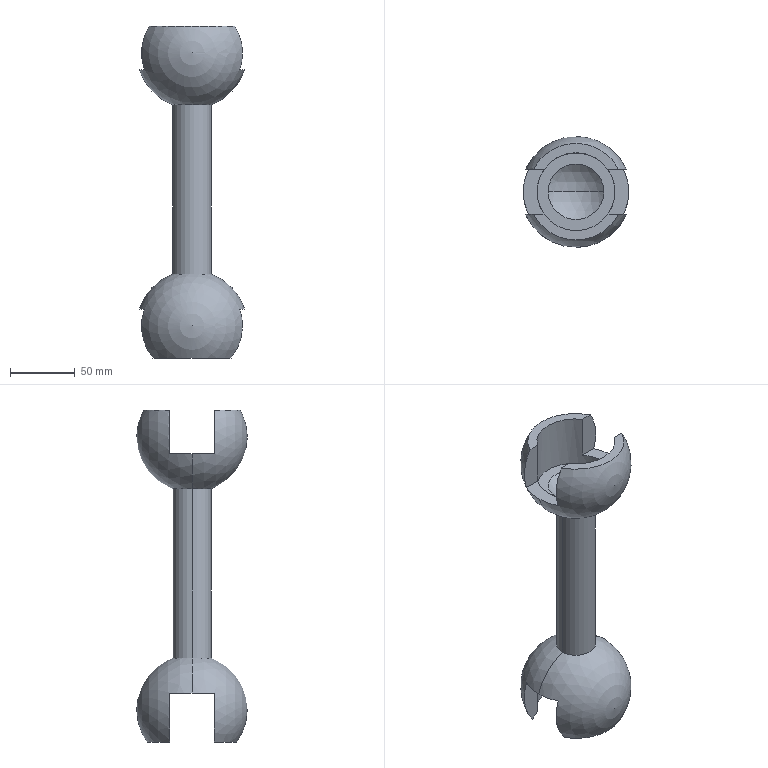Part | SolidWorks | features Chamfer 2, ICE 2, Extrusion 1, MirrorPattern 1, RevCut 1, Revolution 1 | 1 solid | 32 faces | box 80.921 x 85 x 255.451 mm | volume 326390 mm3 | plane 14 | sphere 8 | cylinder 6 | cone 4 | commonest cylinder face diameters 60 x4 30 x2
STEP:
#1=CARTESIAN_POINT('',(15.,0.,65.235));
#2=VERTEX_POINT('',#1);
#3=CARTESIAN_POINT('',(-15.,0.,65.235));
#4=VERTEX_POINT('',#3);
#5=CARTESIAN_POINT('',(0.,0.,65.235));
#6=DIRECTION('',(0.,0.,1.));
#7=DIRECTION('',(1.,0.,0.));
#8=AXIS2_PLACEMENT_3D('',#5,#6,#7);
#9=CIRCLE('',#8,15.);
#10=EDGE_CURVE('',#2,#4,#9,.T.);
#11=ORIENTED_EDGE('',*,*,#10,.T.);
#12=CARTESIAN_POINT('',(-40.46,0.,91.992));
#13=VERTEX_POINT('',#12);
#14=CARTESIAN_POINT('',(0.,0.,105.));
#15=DIRECTION('',(0.,1.,0.));
#16=DIRECTION('',(-1.,0.,0.));
#17=AXIS2_PLACEMENT_3D('',#14,#15,#16);
#18=CIRCLE('',#17,42.5);
#19=EDGE_CURVE('',#4,#13,#18,.T.);
#20=ORIENTED_EDGE('',*,*,#19,.T.);
#21=CARTESIAN_POINT('',(-36.62,17.204,91.992));
#22=VERTEX_POINT('',#21);
#23=CARTESIAN_POINT('',(0.,0.,91.992));
#24=DIRECTION('',(0.,0.,1.));
#25=DIRECTION('',(1.,0.,0.));
#26=AXIS2_PLACEMENT_3D('',#23,#24,#25);
#27=CIRCLE('',#26,40.46);
#28=EDGE_CURVE('',#22,#13,#27,.T.);
#29=ORIENTED_EDGE('',*,*,#28,.F.);
#30=CARTESIAN_POINT('',(-32.854,17.204,125.757));
#31=VERTEX_POINT('',#30);
#32=CARTESIAN_POINT('',(0.,17.204,105.));
#33=DIRECTION('',(0.,-1.,0.));
#34=DIRECTION('',(0.,0.,-1.));
#35=AXIS2_PLACEMENT_3D('',#32,#33,#34);
#36=CIRCLE('',#35,38.862);
#37=EDGE_CURVE('',#31,#22,#36,.T.);
#38=ORIENTED_EDGE('',*,*,#37,.F.);
#39=CARTESIAN_POINT('',(32.854,17.204,125.757));
#40=VERTEX_POINT('',#39);
#41=CARTESIAN_POINT('',(0.,0.,125.757));
#42=DIRECTION('',(0.,0.,-1.));
#43=DIRECTION('',(-1.,0.,0.));
#44=AXIS2_PLACEMENT_3D('',#41,#42,#43);
#45=CIRCLE('',#44,37.086);
#46=EDGE_CURVE('',#31,#40,#45,.T.);
#47=ORIENTED_EDGE('',*,*,#46,.T.);
#48=CARTESIAN_POINT('',(36.62,17.204,91.992));
#49=VERTEX_POINT('',#48);
#50=CARTESIAN_POINT('',(0.,17.204,105.));
#51=DIRECTION('',(0.,-1.,0.));
#52=DIRECTION('',(0.,0.,-1.));
#53=AXIS2_PLACEMENT_3D('',#50,#51,#52);
#54=CIRCLE('',#53,38.862);
#55=EDGE_CURVE('',#49,#40,#54,.T.);
#56=ORIENTED_EDGE('',*,*,#55,.F.);
#57=CARTESIAN_POINT('',(40.46,0.,91.992));
#58=VERTEX_POINT('',#57);
#59=CARTESIAN_POINT('',(0.,0.,91.992));
#60=DIRECTION('',(0.,0.,1.));
#61=DIRECTION('',(1.,0.,0.));
#62=AXIS2_PLACEMENT_3D('',#59,#60,#61);
#63=CIRCLE('',#62,40.46);
#64=EDGE_CURVE('',#58,#49,#63,.T.);
#65=ORIENTED_EDGE('',*,*,#64,.F.);
#66=CARTESIAN_POINT('',(0.,0.,105.));
#67=DIRECTION('',(0.,-1.,0.));
#68=DIRECTION('',(0.,0.,-1.));
#69=AXIS2_PLACEMENT_3D('',#66,#67,#68);
#70=CIRCLE('',#69,42.5);
#71=EDGE_CURVE('',#2,#58,#70,.T.);
#72=ORIENTED_EDGE('',*,*,#71,.F.);
#73=EDGE_LOOP('',(#11,#20,#29,#38,#47,#56,#65,#72));
#74=FACE_OUTER_BOUND('',#73,.T.);
#75=CARTESIAN_POINT('',(0.,0.,105.));
#76=DIRECTION('',(0.,1.,0.));
#77=DIRECTION('',(1.,0.,0.));
#78=AXIS2_PLACEMENT_3D('',#75,#76,#77);
#79=SPHERICAL_SURFACE('',#78,42.5);
#80=ADVANCED_FACE('',(#74),#79,.T.);
#81=CARTESIAN_POINT('',(0.,0.,-75.));
#82=VERTEX_POINT('',#81);
#83=CARTESIAN_POINT('',(-21.424,0.,-84.));
#84=VERTEX_POINT('',#83);
#85=CARTESIAN_POINT('',(0.,0.,-105.));
#86=DIRECTION('',(0.,-1.,0.));
#87=DIRECTION('',(0.,0.,-1.));
#88=AXIS2_PLACEMENT_3D('',#85,#86,#87);
#89=CIRCLE('',#88,30.);
#90=EDGE_CURVE('',#82,#84,#89,.T.);
#91=ORIENTED_EDGE('',*,*,#90,.F.);
#92=CARTESIAN_POINT('',(21.424,0.,-84.));
#93=VERTEX_POINT('',#92);
#94=CARTESIAN_POINT('',(0.,0.,-105.));
#95=DIRECTION('',(0.,1.,0.));
#96=DIRECTION('',(-1.,0.,0.));
#97=AXIS2_PLACEMENT_3D('',#94,#95,#96);
#98=CIRCLE('',#97,30.);
#99=EDGE_CURVE('',#82,#93,#98,.T.);
#100=ORIENTED_EDGE('',*,*,#99,.T.);
#101=CARTESIAN_POINT('',(0.,0.,-84.));
#102=DIRECTION('',(0.,0.,-1.));
#103=DIRECTION('',(1.,0.,0.));
#104=AXIS2_PLACEMENT_3D('',#101,#102,#103);
#105=CIRCLE('',#104,21.424);
#106=EDGE_CURVE('',#93,#84,#105,.T.);
#107=ORIENTED_EDGE('',*,*,#106,.T.);
#108=EDGE_LOOP('',(#91,#100,#107));
#109=FACE_OUTER_BOUND('',#108,.T.);
#110=CARTESIAN_POINT('',(0.,0.,-105.));
#111=DIRECTION('',(0.,1.,0.));
#112=DIRECTION('',(-1.,0.,0.));
#113=AXIS2_PLACEMENT_3D('',#110,#111,#112);
#114=SPHERICAL_SURFACE('',#113,30.);
#115=ADVANCED_FACE('',(#109),#114,.F.);
#116=CARTESIAN_POINT('',(15.,0.,-65.235));
#117=VERTEX_POINT('',#116);
#118=CARTESIAN_POINT('',(-15.,0.,-65.235));
#119=VERTEX_POINT('',#118);
#120=CARTESIAN_POINT('',(0.,0.,-65.235));
#121=DIRECTION('',(0.,0.,-1.));
#122=DIRECTION('',(-1.,0.,0.));
#123=AXIS2_PLACEMENT_3D('',#120,#121,#122);
#124=CIRCLE('',#123,15.);
#125=EDGE_CURVE('',#117,#119,#124,.T.);
#126=ORIENTED_EDGE('',*,*,#125,.T.);
#127=CARTESIAN_POINT('',(-40.46,0.,-91.992));
#128=VERTEX_POINT('',#127);
#129=CARTESIAN_POINT('',(0.,0.,-105.));
#130=DIRECTION('',(0.,-1.,0.));
#131=DIRECTION('',(1.,0.,0.));
#132=AXIS2_PLACEMENT_3D('',#129,#130,#131);
#133=CIRCLE('',#132,42.5);
#134=EDGE_CURVE('',#119,#128,#133,.T.);
#135=ORIENTED_EDGE('',*,*,#134,.T.);
#136=CARTESIAN_POINT('',(-36.62,-17.204,-91.992));
#137=VERTEX_POINT('',#136);
#138=CARTESIAN_POINT('',(0.,0.,-91.992));
#139=DIRECTION('',(0.,0.,1.));
#140=DIRECTION('',(1.,0.,0.));
#141=AXIS2_PLACEMENT_3D('',#138,#139,#140);
#142=CIRCLE('',#141,40.46);
#143=EDGE_CURVE('',#128,#137,#142,.T.);
#144=ORIENTED_EDGE('',*,*,#143,.T.);
#145=CARTESIAN_POINT('',(-30.008,-17.204,-129.694));
#146=VERTEX_POINT('',#145);
#147=CARTESIAN_POINT('',(0.,-17.204,-105.));
#148=DIRECTION('',(0.,1.,0.));
#149=DIRECTION('',(0.,0.,1.));
#150=AXIS2_PLACEMENT_3D('',#147,#148,#149);
#151=CIRCLE('',#150,38.862);
#152=EDGE_CURVE('',#146,#137,#151,.T.);
#153=ORIENTED_EDGE('',*,*,#152,.F.);
#154=CARTESIAN_POINT('',(30.008,-17.204,-129.694));
#155=VERTEX_POINT('',#154);
#156=CARTESIAN_POINT('',(0.,0.,-129.694));
#157=DIRECTION('',(0.,0.,1.));
#158=DIRECTION('',(1.,0.,0.));
#159=AXIS2_PLACEMENT_3D('',#156,#157,#158);
#160=CIRCLE('',#159,34.59);
#161=EDGE_CURVE('',#146,#155,#160,.T.);
#162=ORIENTED_EDGE('',*,*,#161,.T.);
#163=CARTESIAN_POINT('',(36.62,-17.204,-91.992));
#164=VERTEX_POINT('',#163);
#165=CARTESIAN_POINT('',(0.,-17.204,-105.));
#166=DIRECTION('',(0.,1.,0.));
#167=DIRECTION('',(0.,0.,1.));
#168=AXIS2_PLACEMENT_3D('',#165,#166,#167);
#169=CIRCLE('',#168,38.862);
#170=EDGE_CURVE('',#164,#155,#169,.T.);
#171=ORIENTED_EDGE('',*,*,#170,.F.);
#172=CARTESIAN_POINT('',(40.46,0.,-91.992));
#173=VERTEX_POINT('',#172);
#174=CARTESIAN_POINT('',(0.,0.,-91.992));
#175=DIRECTION('',(0.,0.,1.));
#176=DIRECTION('',(1.,0.,0.));
#177=AXIS2_PLACEMENT_3D('',#174,#175,#176);
#178=CIRCLE('',#177,40.46);
#179=EDGE_CURVE('',#164,#173,#178,.T.);
#180=ORIENTED_EDGE('',*,*,#179,.T.);
#181=CARTESIAN_POINT('',(0.,0.,-105.));
#182=DIRECTION('',(0.,1.,0.));
#183=DIRECTION('',(0.,0.,1.));
#184=AXIS2_PLACEMENT_3D('',#181,#182,#183);
#185=CIRCLE('',#184,42.5);
#186=EDGE_CURVE('',#117,#173,#185,.T.);
#187=ORIENTED_EDGE('',*,*,#186,.F.);
#188=EDGE_LOOP('',(#126,#135,#144,#153,#162,#171,#180,#187));
#189=FACE_OUTER_BOUND('',#188,.T.);
#190=CARTESIAN_POINT('',(0.,0.,-105.));
#191=DIRECTION('',(0.,-1.,0.));
#192=DIRECTION('',(1.,0.,0.));
#193=AXIS2_PLACEMENT_3D('',#190,#191,#192);
#194=SPHERICAL_SURFACE('',#193,42.5);
#195=ADVANCED_FACE('',(#189),#194,.T.);
#196=CARTESIAN_POINT('',(-30.,0.,-84.));
#197=VERTEX_POINT('',#196);
#198=CARTESIAN_POINT('',(30.,0.,-84.));
#199=VERTEX_POINT('',#198);
#200=CARTESIAN_POINT('',(0.,0.,-84.));
#201=DIRECTION('',(0.,0.,1.));
#202=DIRECTION('',(1.,0.,0.));
#203=AXIS2_PLACEMENT_3D('',#200,#201,#202);
#204=CIRCLE('',#203,30.);
#205=EDGE_CURVE('',#197,#199,#204,.T.);
#206=ORIENTED_EDGE('',*,*,#205,.T.);
#207=CARTESIAN_POINT('',(30.,0.,-91.992));
#208=VERTEX_POINT('',#207);
#209=CARTESIAN_POINT('',(30.,0.,-84.));
#210=DIRECTION('',(0.,0.,-1.));
#211=VECTOR('',#210,1000.);
#212=LINE('',#209,#211);
#213=EDGE_CURVE('',#199,#208,#212,.T.);
#214=ORIENTED_EDGE('',*,*,#213,.T.);
#215=CARTESIAN_POINT('',(24.577,-17.204,-91.992));
#216=VERTEX_POINT('',#215);
#217=CARTESIAN_POINT('',(0.,0.,-91.992));
#218=DIRECTION('',(0.,0.,1.));
#219=DIRECTION('',(1.,0.,0.));
#220=AXIS2_PLACEMENT_3D('',#217,#218,#219);
#221=CIRCLE('',#220,30.);
#222=EDGE_CURVE('',#216,#208,#221,.T.);
#223=ORIENTED_EDGE('',*,*,#222,.F.);
#224=CARTESIAN_POINT('',(24.577,-17.204,-125.104));
#225=VERTEX_POINT('',#224);
#226=CARTESIAN_POINT('',(24.577,-17.204,-84.));
#227=DIRECTION('',(0.,0.,-1.));
#228=VECTOR('',#227,1000.);
#229=LINE('',#226,#228);
#230=EDGE_CURVE('',#216,#225,#229,.T.);
#231=ORIENTED_EDGE('',*,*,#230,.T.);
#232=CARTESIAN_POINT('',(-24.577,-17.204,-125.104));
#233=VERTEX_POINT('',#232);
#234=CARTESIAN_POINT('',(0.,0.,-125.104));
#235=DIRECTION('',(0.,0.,-1.));
#236=DIRECTION('',(1.,0.,0.));
#237=AXIS2_PLACEMENT_3D('',#234,#235,#236);
#238=CIRCLE('',#237,30.);
#239=EDGE_CURVE('',#225,#233,#238,.T.);
#240=ORIENTED_EDGE('',*,*,#239,.T.);
#241=CARTESIAN_POINT('',(-24.577,-17.204,-91.992));
#242=VERTEX_POINT('',#241);
#243=CARTESIAN_POINT('',(-24.577,-17.204,-84.));
#244=DIRECTION('',(0.,0.,1.));
#245=VECTOR('',#244,1000.);
#246=LINE('',#243,#245);
#247=EDGE_CURVE('',#233,#242,#246,.T.);
#248=ORIENTED_EDGE('',*,*,#247,.T.);
#249=CARTESIAN_POINT('',(-30.,0.,-91.992));
#250=VERTEX_POINT('',#249);
#251=CARTESIAN_POINT('',(0.,0.,-91.992));
#252=DIRECTION('',(0.,0.,1.));
#253=DIRECTION('',(1.,0.,0.));
#254=AXIS2_PLACEMENT_3D('',#251,#252,#253);
#255=CIRCLE('',#254,30.);
#256=EDGE_CURVE('',#250,#242,#255,.T.);
#257=ORIENTED_EDGE('',*,*,#256,.F.);
#258=CARTESIAN_POINT('',(-30.,0.,-84.));
#259=DIRECTION('',(0.,0.,-1.));
#260=VECTOR('',#259,1000.);
#261=LINE('',#258,#260);
#262=EDGE_CURVE('',#197,#250,#261,.T.);
#263=ORIENTED_EDGE('',*,*,#262,.F.);
#264=EDGE_LOOP('',(#206,#214,#223,#231,#240,#248,#257,#263));
#265=FACE_OUTER_BOUND('',#264,.T.);
#266=CARTESIAN_POINT('',(0.,0.,-84.));
#267=DIRECTION('',(0.,0.,-1.));
#268=DIRECTION('',(-1.,0.,0.));
#269=AXIS2_PLACEMENT_3D('',#266,#267,#268);
#270=CYLINDRICAL_SURFACE('',#269,30.);
#271=ADVANCED_FACE('',(#265),#270,.F.);
#272=ORIENTED_EDGE('',*,*,#10,.F.);
#273=CARTESIAN_POINT('',(15.,0.,80.));
#274=DIRECTION('',(0.,0.,-1.));
#275=VECTOR('',#274,1000.);
#276=LINE('',#273,#275);
#277=EDGE_CURVE('',#2,#117,#276,.T.);
#278=ORIENTED_EDGE('',*,*,#277,.T.);
#279=CARTESIAN_POINT('',(0.,0.,-65.235));
#280=DIRECTION('',(0.,0.,-1.));
#281=DIRECTION('',(-1.,0.,0.));
#282=AXIS2_PLACEMENT_3D('',#279,#280,#281);
#283=CIRCLE('',#282,15.);
#284=EDGE_CURVE('',#119,#117,#283,.T.);
#285=ORIENTED_EDGE('',*,*,#284,.F.);
#286=CARTESIAN_POINT('',(-15.,0.,80.));
#287=DIRECTION('',(0.,0.,-1.));
#288=VECTOR('',#287,1000.);
#289=LINE('',#286,#288);
#290=EDGE_CURVE('',#4,#119,#289,.T.);
#291=ORIENTED_EDGE('',*,*,#290,.F.);
#292=EDGE_LOOP('',(#272,#278,#285,#291));
#293=FACE_OUTER_BOUND('',#292,.T.);
#294=CARTESIAN_POINT('',(0.,0.,80.));
#295=DIRECTION('',(0.,0.,-1.));
#296=DIRECTION('',(-1.,0.,0.));
#297=AXIS2_PLACEMENT_3D('',#294,#295,#296);
#298=CYLINDRICAL_SURFACE('',#297,15.);
#299=ADVANCED_FACE('',(#293),#298,.T.);
#300=CARTESIAN_POINT('',(-30.,0.,84.));
#301=VERTEX_POINT('',#300);
#302=CARTESIAN_POINT('',(30.,0.,84.));
#303=VERTEX_POINT('',#302);
#304=CARTESIAN_POINT('',(0.,0.,84.));
#305=DIRECTION('',(0.,0.,1.));
#306=DIRECTION('',(1.,0.,0.));
#307=AXIS2_PLACEMENT_3D('',#304,#305,#306);
#308=CIRCLE('',#307,30.);
#309=EDGE_CURVE('',#301,#303,#308,.T.);
#310=ORIENTED_EDGE('',*,*,#309,.F.);
#311=CARTESIAN_POINT('',(-30.,0.,91.992));
#312=VERTEX_POINT('',#311);
#313=CARTESIAN_POINT('',(-30.,0.,84.));
#314=DIRECTION('',(0.,0.,1.));
#315=VECTOR('',#314,1000.);
#316=LINE('',#313,#315);
#317=EDGE_CURVE('',#301,#312,#316,.T.);
#318=ORIENTED_EDGE('',*,*,#317,.T.);
#319=CARTESIAN_POINT('',(-24.577,-17.204,91.992));
#320=VERTEX_POINT('',#319);
#321=CARTESIAN_POINT('',(0.,0.,91.992));
#322=DIRECTION('',(0.,0.,-1.));
#323=DIRECTION('',(1.,0.,0.));
#324=AXIS2_PLACEMENT_3D('',#321,#322,#323);
#325=CIRCLE('',#324,30.);
#326=EDGE_CURVE('',#320,#312,#325,.T.);
#327=ORIENTED_EDGE('',*,*,#326,.F.);
#328=CARTESIAN_POINT('',(-24.577,-17.204,125.749));
#329=VERTEX_POINT('',#328);
#330=CARTESIAN_POINT('',(-24.577,-17.204,84.));
#331=DIRECTION('',(0.,0.,1.));
#332=VECTOR('',#331,1000.);
#333=LINE('',#330,#332);
#334=EDGE_CURVE('',#320,#329,#333,.T.);
#335=ORIENTED_EDGE('',*,*,#334,.T.);
#336=CARTESIAN_POINT('',(24.577,-17.204,125.749));
#337=VERTEX_POINT('',#336);
#338=CARTESIAN_POINT('',(0.,0.,125.749));
#339=DIRECTION('',(0.,0.,1.));
#340=DIRECTION('',(-1.,0.,0.));
#341=AXIS2_PLACEMENT_3D('',#338,#339,#340);
#342=CIRCLE('',#341,30.);
#343=EDGE_CURVE('',#329,#337,#342,.T.);
#344=ORIENTED_EDGE('',*,*,#343,.T.);
#345=CARTESIAN_POINT('',(24.577,-17.204,91.992));
#346=VERTEX_POINT('',#345);
#347=CARTESIAN_POINT('',(24.577,-17.204,84.));
#348=DIRECTION('',(0.,0.,-1.));
#349=VECTOR('',#348,1000.);
#350=LINE('',#347,#349);
#351=EDGE_CURVE('',#337,#346,#350,.T.);
#352=ORIENTED_EDGE('',*,*,#351,.T.);
#353=CARTESIAN_POINT('',(30.,0.,91.992));
#354=VERTEX_POINT('',#353);
#355=CARTESIAN_POINT('',(0.,0.,91.992));
#356=DIRECTION('',(0.,0.,-1.));
#357=DIRECTION('',(1.,0.,0.));
#358=AXIS2_PLACEMENT_3D('',#355,#356,#357);
#359=CIRCLE('',#358,30.);
#360=EDGE_CURVE('',#354,#346,#359,.T.);
#361=ORIENTED_EDGE('',*,*,#360,.F.);
#362=CARTESIAN_POINT('',(30.,0.,84.));
#363=DIRECTION('',(0.,0.,1.));
#364=VECTOR('',#363,1000.);
#365=LINE('',#362,#364);
#366=EDGE_CURVE('',#303,#354,#365,.T.);
#367=ORIENTED_EDGE('',*,*,#366,.F.);
#368=EDGE_LOOP('',(#310,#318,#327,#335,#344,#352,#361,#367));
#369=FACE_OUTER_BOUND('',#368,.T.);
#370=CARTESIAN_POINT('',(0.,0.,84.));
#371=DIRECTION('',(0.,0.,1.));
#372=DIRECTION('',(1.,0.,0.));
#373=AXIS2_PLACEMENT_3D('',#370,#371,#372);
#374=CYLINDRICAL_SURFACE('',#373,30.);
#375=ADVANCED_FACE('',(#369),#374,.F.);
#376=CARTESIAN_POINT('',(0.,0.,75.));
#377=VERTEX_POINT('',#376);
#378=CARTESIAN_POINT('',(-21.424,0.,84.));
#379=VERTEX_POINT('',#378);
#380=CARTESIAN_POINT('',(0.,0.,105.));
#381=DIRECTION('',(0.,1.,0.));
#382=DIRECTION('',(0.,0.,1.));
#383=AXIS2_PLACEMENT_3D('',#380,#381,#382);
#384=CIRCLE('',#383,30.);
#385=EDGE_CURVE('',#377,#379,#384,.T.);
#386=ORIENTED_EDGE('',*,*,#385,.F.);
#387=CARTESIAN_POINT('',(21.424,0.,84.));
#388=VERTEX_POINT('',#387);
#389=CARTESIAN_POINT('',(0.,0.,105.));
#390=DIRECTION('',(0.,-1.,0.));
#391=DIRECTION('',(1.,0.,0.));
#392=AXIS2_PLACEMENT_3D('',#389,#390,#391);
#393=CIRCLE('',#392,30.);
#394=EDGE_CURVE('',#377,#388,#393,.T.);
#395=ORIENTED_EDGE('',*,*,#394,.T.);
#396=CARTESIAN_POINT('',(0.,0.,84.));
#397=DIRECTION('',(0.,0.,1.));
#398=DIRECTION('',(-1.,0.,0.));
#399=AXIS2_PLACEMENT_3D('',#396,#397,#398);
#400=CIRCLE('',#399,21.424);
#401=EDGE_CURVE('',#388,#379,#400,.T.);
#402=ORIENTED_EDGE('',*,*,#401,.T.);
#403=EDGE_LOOP('',(#386,#395,#402));
#404=FACE_OUTER_BOUND('',#403,.T.);
#405=CARTESIAN_POINT('',(0.,0.,105.));
#406=DIRECTION('',(0.,-1.,0.));
#407=DIRECTION('',(-1.,0.,0.));
#408=AXIS2_PLACEMENT_3D('',#405,#406,#407);
#409=SPHERICAL_SURFACE('',#408,30.);
#410=ADVANCED_FACE('',(#404),#409,.F.);
#411=ORIENTED_EDGE('',*,*,#394,.F.);
#412=ORIENTED_EDGE('',*,*,#385,.T.);
#413=CARTESIAN_POINT('',(0.,0.,84.));
#414=DIRECTION('',(0.,0.,1.));
#415=DIRECTION('',(-1.,0.,0.));
#416=AXIS2_PLACEMENT_3D('',#413,#414,#415);
#417=CIRCLE('',#416,21.424);
#418=EDGE_CURVE('',#379,#388,#417,.T.);
#419=ORIENTED_EDGE('',*,*,#418,.T.);
#420=EDGE_LOOP('',(#411,#412,#419));
#421=FACE_OUTER_BOUND('',#420,.T.);
#422=CARTESIAN_POINT('',(0.,0.,105.));
#423=DIRECTION('',(0.,-1.,0.));
#424=DIRECTION('',(-1.,0.,0.));
#425=AXIS2_PLACEMENT_3D('',#422,#423,#424);
#426=SPHERICAL_SURFACE('',#425,30.);
#427=ADVANCED_FACE('',(#421),#426,.F.);
#428=ORIENTED_EDGE('',*,*,#317,.F.);
#429=CARTESIAN_POINT('',(0.,0.,84.));
#430=DIRECTION('',(0.,0.,1.));
#431=DIRECTION('',(1.,0.,0.));
#432=AXIS2_PLACEMENT_3D('',#429,#430,#431);
#433=CIRCLE('',#432,30.);
#434=EDGE_CURVE('',#303,#301,#433,.T.);
#435=ORIENTED_EDGE('',*,*,#434,.F.);
#436=ORIENTED_EDGE('',*,*,#366,.T.);
#437=CARTESIAN_POINT('',(24.577,17.204,91.992));
#438=VERTEX_POINT('',#437);
#439=CARTESIAN_POINT('',(0.,0.,91.992));
#440=DIRECTION('',(0.,0.,-1.));
#441=DIRECTION('',(1.,0.,0.));
#442=AXIS2_PLACEMENT_3D('',#439,#440,#441);
#443=CIRCLE('',#442,30.);
#444=EDGE_CURVE('',#438,#354,#443,.T.);
#445=ORIENTED_EDGE('',*,*,#444,.F.);
#446=CARTESIAN_POINT('',(24.577,17.204,125.749));
#447=VERTEX_POINT('',#446);
#448=CARTESIAN_POINT('',(24.577,17.204,84.));
#449=DIRECTION('',(0.,0.,-1.));
#450=VECTOR('',#449,1000.);
#451=LINE('',#448,#450);
#452=EDGE_CURVE('',#447,#438,#451,.T.);
#453=ORIENTED_EDGE('',*,*,#452,.F.);
#454=CARTESIAN_POINT('',(-24.577,17.204,125.749));
#455=VERTEX_POINT('',#454);
#456=CARTESIAN_POINT('',(0.,0.,125.749));
#457=DIRECTION('',(0.,0.,1.));
#458=DIRECTION('',(-1.,0.,0.));
#459=AXIS2_PLACEMENT_3D('',#456,#457,#458);
#460=CIRCLE('',#459,30.);
#461=EDGE_CURVE('',#447,#455,#460,.T.);
#462=ORIENTED_EDGE('',*,*,#461,.T.);
#463=CARTESIAN_POINT('',(-24.577,17.204,91.992));
#464=VERTEX_POINT('',#463);
#465=CARTESIAN_POINT('',(-24.577,17.204,84.));
#466=DIRECTION('',(0.,0.,1.));
#467=VECTOR('',#466,1000.);
#468=LINE('',#465,#467);
#469=EDGE_CURVE('',#464,#455,#468,.T.);
#470=ORIENTED_EDGE('',*,*,#469,.F.);
#471=CARTESIAN_POINT('',(0.,0.,91.992));
#472=DIRECTION('',(0.,0.,-1.));
#473=DIRECTION('',(1.,0.,0.));
#474=AXIS2_PLACEMENT_3D('',#471,#472,#473);
#475=CIRCLE('',#474,30.);
#476=EDGE_CURVE('',#312,#464,#475,.T.);
#477=ORIENTED_EDGE('',*,*,#476,.F.);
#478=EDGE_LOOP('',(#428,#435,#436,#445,#453,#462,#470,#477));
#479=FACE_OUTER_BOUND('',#478,.T.);
#480=CARTESIAN_POINT('',(0.,0.,84.));
#481=DIRECTION('',(0.,0.,1.));
#482=DIRECTION('',(1.,0.,0.));
#483=AXIS2_PLACEMENT_3D('',#480,#481,#482);
#484=CYLINDRICAL_SURFACE('',#483,30.);
#485=ADVANCED_FACE('',(#479),#484,.F.);
#486=ORIENTED_EDGE('',*,*,#434,.T.);
#487=ORIENTED_EDGE('',*,*,#309,.T.);
#488=EDGE_LOOP('',(#486,#487));
#489=FACE_OUTER_BOUND('',#488,.T.);
#490=ORIENTED_EDGE('',*,*,#418,.F.);
#491=ORIENTED_EDGE('',*,*,#401,.F.);
#492=EDGE_LOOP('',(#490,#491));
#493=FACE_BOUND('',#492,.T.);
#494=CARTESIAN_POINT('',(0.,0.,84.));
#495=DIRECTION('',(0.,0.,-1.));
#496=DIRECTION('',(1.,0.,0.));
#497=AXIS2_PLACEMENT_3D('',#494,#495,#496);
#498=PLANE('',#497);
#499=ADVANCED_FACE('',(#489,#493),#498,.F.);
#500=ORIENTED_EDGE('',*,*,#277,.F.);
#501=CARTESIAN_POINT('',(0.,0.,65.235));
#502=DIRECTION('',(0.,0.,1.));
#503=DIRECTION('',(1.,0.,0.));
#504=AXIS2_PLACEMENT_3D('',#501,#502,#503);
#505=CIRCLE('',#504,15.);
#506=EDGE_CURVE('',#4,#2,#505,.T.);
#507=ORIENTED_EDGE('',*,*,#506,.F.);
#508=ORIENTED_EDGE('',*,*,#290,.T.);
#509=ORIENTED_EDGE('',*,*,#125,.F.);
#510=EDGE_LOOP('',(#500,#507,#508,#509));
#511=FACE_OUTER_BOUND('',#510,.T.);
#512=CARTESIAN_POINT('',(0.,0.,80.));
#513=DIRECTION('',(0.,0.,-1.));
#514=DIRECTION('',(-1.,0.,0.));
#515=AXIS2_PLACEMENT_3D('',#512,#513,#514);
#516=CYLINDRICAL_SURFACE('',#515,15.);
#517=ADVANCED_FACE('',(#511),#516,.T.);
#518=ORIENTED_EDGE('',*,*,#213,.F.);
#519=CARTESIAN_POINT('',(0.,0.,-84.));
#520=DIRECTION('',(0.,0.,1.));
#521=DIRECTION('',(1.,0.,0.));
#522=AXIS2_PLACEMENT_3D('',#519,#520,#521);
#523=CIRCLE('',#522,30.);
#524=EDGE_CURVE('',#199,#197,#523,.T.);
#525=ORIENTED_EDGE('',*,*,#524,.T.);
#526=ORIENTED_EDGE('',*,*,#262,.T.);
#527=CARTESIAN_POINT('',(-24.577,17.204,-91.992));
#528=VERTEX_POINT('',#527);
#529=CARTESIAN_POINT('',(0.,0.,-91.992));
#530=DIRECTION('',(0.,0.,1.));
#531=DIRECTION('',(1.,0.,0.));
#532=AXIS2_PLACEMENT_3D('',#529,#530,#531);
#533=CIRCLE('',#532,30.);
#534=EDGE_CURVE('',#528,#250,#533,.T.);
#535=ORIENTED_EDGE('',*,*,#534,.F.);
#536=CARTESIAN_POINT('',(-24.577,17.204,-125.104));
#537=VERTEX_POINT('',#536);
#538=CARTESIAN_POINT('',(-24.577,17.204,-84.));
#539=DIRECTION('',(0.,0.,1.));
#540=VECTOR('',#539,1000.);
#541=LINE('',#538,#540);
#542=EDGE_CURVE('',#537,#528,#541,.T.);
#543=ORIENTED_EDGE('',*,*,#542,.F.);
#544=CARTESIAN_POINT('',(24.577,17.204,-125.104));
#545=VERTEX_POINT('',#544);
#546=CARTESIAN_POINT('',(0.,0.,-125.104));
#547=DIRECTION('',(0.,0.,-1.));
#548=DIRECTION('',(1.,0.,0.));
#549=AXIS2_PLACEMENT_3D('',#546,#547,#548);
#550=CIRCLE('',#549,30.);
#551=EDGE_CURVE('',#537,#545,#550,.T.);
#552=ORIENTED_EDGE('',*,*,#551,.T.);
#553=CARTESIAN_POINT('',(24.577,17.204,-91.992));
#554=VERTEX_POINT('',#553);
#555=CARTESIAN_POINT('',(24.577,17.204,-84.));
#556=DIRECTION('',(0.,0.,-1.));
#557=VECTOR('',#556,1000.);
#558=LINE('',#555,#557);
#559=EDGE_CURVE('',#554,#545,#558,.T.);
#560=ORIENTED_EDGE('',*,*,#559,.F.);
#561=CARTESIAN_POINT('',(0.,0.,-91.992));
#562=DIRECTION('',(0.,0.,1.));
#563=DIRECTION('',(1.,0.,0.));
#564=AXIS2_PLACEMENT_3D('',#561,#562,#563);
#565=CIRCLE('',#564,30.);
#566=EDGE_CURVE('',#208,#554,#565,.T.);
#567=ORIENTED_EDGE('',*,*,#566,.F.);
#568=EDGE_LOOP('',(#518,#525,#526,#535,#543,#552,#560,#567));
#569=FACE_OUTER_BOUND('',#568,.T.);
#570=CARTESIAN_POINT('',(0.,0.,-84.));
#571=DIRECTION('',(0.,0.,-1.));
#572=DIRECTION('',(-1.,0.,0.));
#573=AXIS2_PLACEMENT_3D('',#570,#571,#572);
#574=CYLINDRICAL_SURFACE('',#573,30.);
#575=ADVANCED_FACE('',(#569),#574,.F.);
#576=ORIENTED_EDGE('',*,*,#134,.F.);
#577=ORIENTED_EDGE('',*,*,#284,.T.);
#578=ORIENTED_EDGE('',*,*,#186,.T.);
#579=CARTESIAN_POINT('',(36.62,17.204,-91.992));
#580=VERTEX_POINT('',#579);
#581=CARTESIAN_POINT('',(0.,0.,-91.992));
#582=DIRECTION('',(0.,0.,1.));
#583=DIRECTION('',(1.,0.,0.));
#584=AXIS2_PLACEMENT_3D('',#581,#582,#583);
#585=CIRCLE('',#584,40.46);
#586=EDGE_CURVE('',#173,#580,#585,.T.);
#587=ORIENTED_EDGE('',*,*,#586,.T.);
#588=CARTESIAN_POINT('',(30.008,17.204,-129.694));
#589=VERTEX_POINT('',#588);
#590=CARTESIAN_POINT('',(0.,17.204,-105.));
#591=DIRECTION('',(0.,1.,0.));
#592=DIRECTION('',(0.,0.,1.));
#593=AXIS2_PLACEMENT_3D('',#590,#591,#592);
#594=CIRCLE('',#593,38.862);
#595=EDGE_CURVE('',#580,#589,#594,.T.);
#596=ORIENTED_EDGE('',*,*,#595,.T.);
#597=CARTESIAN_POINT('',(-30.008,17.204,-129.694));
#598=VERTEX_POINT('',#597);
#599=CARTESIAN_POINT('',(0.,0.,-129.694));
#600=DIRECTION('',(0.,0.,1.));
#601=DIRECTION('',(1.,0.,0.));
#602=AXIS2_PLACEMENT_3D('',#599,#600,#601);
#603=CIRCLE('',#602,34.59);
#604=EDGE_CURVE('',#589,#598,#603,.T.);
#605=ORIENTED_EDGE('',*,*,#604,.T.);
#606=CARTESIAN_POINT('',(-36.62,17.204,-91.992));
#607=VERTEX_POINT('',#606);
#608=CARTESIAN_POINT('',(0.,17.204,-105.));
#609=DIRECTION('',(0.,1.,0.));
#610=DIRECTION('',(0.,0.,1.));
#611=AXIS2_PLACEMENT_3D('',#608,#609,#610);
#612=CIRCLE('',#611,38.862);
#613=EDGE_CURVE('',#598,#607,#612,.T.);
#614=ORIENTED_EDGE('',*,*,#613,.T.);
#615=CARTESIAN_POINT('',(0.,0.,-91.992));
#616=DIRECTION('',(0.,0.,1.));
#617=DIRECTION('',(1.,0.,0.));
#618=AXIS2_PLACEMENT_3D('',#615,#616,#617);
#619=CIRCLE('',#618,40.46);
#620=EDGE_CURVE('',#607,#128,#619,.T.);
#621=ORIENTED_EDGE('',*,*,#620,.T.);
#622=EDGE_LOOP('',(#576,#577,#578,#587,#596,#605,#614,#621));
#623=FACE_OUTER_BOUND('',#622,.T.);
#624=CARTESIAN_POINT('',(0.,0.,-105.));
#625=DIRECTION('',(0.,-1.,0.));
#626=DIRECTION('',(1.,0.,0.));
#627=AXIS2_PLACEMENT_3D('',#624,#625,#626);
#628=SPHERICAL_SURFACE('',#627,42.5);
#629=ADVANCED_FACE('',(#623),#628,.T.);
#630=ORIENTED_EDGE('',*,*,#99,.F.);
#631=ORIENTED_EDGE('',*,*,#90,.T.);
#632=CARTESIAN_POINT('',(0.,0.,-84.));
#633=DIRECTION('',(0.,0.,-1.));
#634=DIRECTION('',(1.,0.,0.));
#635=AXIS2_PLACEMENT_3D('',#632,#633,#634);
#636=CIRCLE('',#635,21.424);
#637=EDGE_CURVE('',#84,#93,#636,.T.);
#638=ORIENTED_EDGE('',*,*,#637,.T.);
#639=EDGE_LOOP('',(#630,#631,#638));
#640=FACE_OUTER_BOUND('',#639,.T.);
#641=CARTESIAN_POINT('',(0.,0.,-105.));
#642=DIRECTION('',(0.,1.,0.));
#643=DIRECTION('',(-1.,0.,0.));
#644=AXIS2_PLACEMENT_3D('',#641,#642,#643);
#645=SPHERICAL_SURFACE('',#644,30.);
#646=ADVANCED_FACE('',(#640),#645,.F.);
#647=ORIENTED_EDGE('',*,*,#205,.F.);
#648=ORIENTED_EDGE('',*,*,#524,.F.);
#649=EDGE_LOOP('',(#647,#648));
#650=FACE_OUTER_BOUND('',#649,.T.);
#651=ORIENTED_EDGE('',*,*,#637,.F.);
#652=ORIENTED_EDGE('',*,*,#106,.F.);
#653=EDGE_LOOP('',(#651,#652));
#654=FACE_BOUND('',#653,.T.);
#655=CARTESIAN_POINT('',(0.,0.,-84.));
#656=DIRECTION('',(0.,0.,1.));
#657=DIRECTION('',(1.,0.,0.));
#658=AXIS2_PLACEMENT_3D('',#655,#656,#657);
#659=PLANE('',#658);
#660=ADVANCED_FACE('',(#650,#654),#659,.F.);
#661=ORIENTED_EDGE('',*,*,#613,.F.);
#662=CARTESIAN_POINT('',(-30.008,17.204,-129.694));
#663=CARTESIAN_POINT('',(-28.217,17.204,-128.14));
#664=CARTESIAN_POINT('',(-26.411,17.204,-126.606));
#665=CARTESIAN_POINT('',(-24.577,17.204,-125.104));
#666=B_SPLINE_CURVE_WITH_KNOTS('',3,(#662,#663,#664,#665),.UNSPECIFIED.,.F.,.F.,(4,4),(0.,0.007111),.UNSPECIFIED.);
#667=EDGE_CURVE('',#598,#537,#666,.T.);
#668=ORIENTED_EDGE('',*,*,#667,.T.);
#669=ORIENTED_EDGE('',*,*,#542,.T.);
#670=CARTESIAN_POINT('',(-75.5,17.204,-91.992));
#671=DIRECTION('',(1.,0.,0.));
#672=VECTOR('',#671,1000.);
#673=LINE('',#670,#672);
#674=EDGE_CURVE('',#607,#528,#673,.T.);
#675=ORIENTED_EDGE('',*,*,#674,.F.);
#676=EDGE_LOOP('',(#661,#668,#669,#675));
#677=FACE_OUTER_BOUND('',#676,.T.);
#678=CARTESIAN_POINT('',(-75.5,17.204,-178.216));
#679=DIRECTION('',(0.,1.,0.));
#680=DIRECTION('',(0.,0.,1.));
#681=AXIS2_PLACEMENT_3D('',#678,#679,#680);
#682=PLANE('',#681);
#683=ADVANCED_FACE('',(#677),#682,.F.);
#684=ORIENTED_EDGE('',*,*,#534,.T.);
#685=ORIENTED_EDGE('',*,*,#256,.T.);
#686=CARTESIAN_POINT('',(-75.5,-17.204,-91.992));
#687=DIRECTION('',(1.,0.,0.));
#688=VECTOR('',#687,1000.);
#689=LINE('',#686,#688);
#690=EDGE_CURVE('',#137,#242,#689,.T.);
#691=ORIENTED_EDGE('',*,*,#690,.F.);
#692=ORIENTED_EDGE('',*,*,#143,.F.);
#693=ORIENTED_EDGE('',*,*,#620,.F.);
#694=ORIENTED_EDGE('',*,*,#674,.T.);
#695=EDGE_LOOP('',(#684,#685,#691,#692,#693,#694));
#696=FACE_OUTER_BOUND('',#695,.T.);
#697=CARTESIAN_POINT('',(-75.5,17.204,-91.992));
#698=DIRECTION('',(0.,0.,1.));
#699=DIRECTION('',(1.,0.,0.));
#700=AXIS2_PLACEMENT_3D('',#697,#698,#699);
#701=PLANE('',#700);
#702=ADVANCED_FACE('',(#696),#701,.F.);
#703=ORIENTED_EDGE('',*,*,#247,.F.);
#704=CARTESIAN_POINT('',(-24.577,-17.204,-125.104));
#705=CARTESIAN_POINT('',(-26.411,-17.204,-126.606));
#706=CARTESIAN_POINT('',(-28.217,-17.204,-128.14));
#707=CARTESIAN_POINT('',(-30.008,-17.204,-129.694));
#708=B_SPLINE_CURVE_WITH_KNOTS('',3,(#704,#705,#706,#707),.UNSPECIFIED.,.F.,.F.,(4,4),(0.,0.007111),.UNSPECIFIED.);
#709=EDGE_CURVE('',#233,#146,#708,.T.);
#710=ORIENTED_EDGE('',*,*,#709,.T.);
#711=ORIENTED_EDGE('',*,*,#152,.T.);
#712=ORIENTED_EDGE('',*,*,#690,.T.);
#713=EDGE_LOOP('',(#703,#710,#711,#712));
#714=FACE_OUTER_BOUND('',#713,.T.);
#715=CARTESIAN_POINT('',(-75.5,-17.204,-178.216));
#716=DIRECTION('',(0.,1.,0.));
#717=DIRECTION('',(0.,0.,1.));
#718=AXIS2_PLACEMENT_3D('',#715,#716,#717);
#719=PLANE('',#718);
#720=ADVANCED_FACE('',(#714),#719,.T.);
#721=ORIENTED_EDGE('',*,*,#170,.T.);
#722=CARTESIAN_POINT('',(30.008,-17.204,-129.694));
#723=CARTESIAN_POINT('',(28.217,-17.204,-128.14));
#724=CARTESIAN_POINT('',(26.411,-17.204,-126.606));
#725=CARTESIAN_POINT('',(24.577,-17.204,-125.104));
#726=B_SPLINE_CURVE_WITH_KNOTS('',3,(#722,#723,#724,#725),.UNSPECIFIED.,.F.,.F.,(4,4),(0.,0.007111),.UNSPECIFIED.);
#727=EDGE_CURVE('',#155,#225,#726,.T.);
#728=ORIENTED_EDGE('',*,*,#727,.T.);
#729=ORIENTED_EDGE('',*,*,#230,.F.);
#730=CARTESIAN_POINT('',(-75.5,-17.204,-91.992));
#731=DIRECTION('',(1.,0.,0.));
#732=VECTOR('',#731,1000.);
#733=LINE('',#730,#732);
#734=EDGE_CURVE('',#216,#164,#733,.T.);
#735=ORIENTED_EDGE('',*,*,#734,.T.);
#736=EDGE_LOOP('',(#721,#728,#729,#735));
#737=FACE_OUTER_BOUND('',#736,.T.);
#738=CARTESIAN_POINT('',(-75.5,-17.204,-178.216));
#739=DIRECTION('',(0.,1.,0.));
#740=DIRECTION('',(0.,0.,1.));
#741=AXIS2_PLACEMENT_3D('',#738,#739,#740);
#742=PLANE('',#741);
#743=ADVANCED_FACE('',(#737),#742,.T.);
#744=ORIENTED_EDGE('',*,*,#222,.T.);
#745=ORIENTED_EDGE('',*,*,#566,.T.);
#746=CARTESIAN_POINT('',(-75.5,17.204,-91.992));
#747=DIRECTION('',(1.,0.,0.));
#748=VECTOR('',#747,1000.);
#749=LINE('',#746,#748);
#750=EDGE_CURVE('',#554,#580,#749,.T.);
#751=ORIENTED_EDGE('',*,*,#750,.T.);
#752=ORIENTED_EDGE('',*,*,#586,.F.);
#753=ORIENTED_EDGE('',*,*,#179,.F.);
#754=ORIENTED_EDGE('',*,*,#734,.F.);
#755=EDGE_LOOP('',(#744,#745,#751,#752,#753,#754));
#756=FACE_OUTER_BOUND('',#755,.T.);
#757=CARTESIAN_POINT('',(-75.5,17.204,-91.992));
#758=DIRECTION('',(0.,0.,1.));
#759=DIRECTION('',(1.,0.,0.));
#760=AXIS2_PLACEMENT_3D('',#757,#758,#759);
#761=PLANE('',#760);
#762=ADVANCED_FACE('',(#756),#761,.F.);
#763=ORIENTED_EDGE('',*,*,#559,.T.);
#764=CARTESIAN_POINT('',(24.577,17.204,-125.104));
#765=CARTESIAN_POINT('',(26.411,17.204,-126.606));
#766=CARTESIAN_POINT('',(28.217,17.204,-128.14));
#767=CARTESIAN_POINT('',(30.008,17.204,-129.694));
#768=B_SPLINE_CURVE_WITH_KNOTS('',3,(#764,#765,#766,#767),.UNSPECIFIED.,.F.,.F.,(4,4),(0.,0.007111),.UNSPECIFIED.);
#769=EDGE_CURVE('',#545,#589,#768,.T.);
#770=ORIENTED_EDGE('',*,*,#769,.T.);
#771=ORIENTED_EDGE('',*,*,#595,.F.);
#772=ORIENTED_EDGE('',*,*,#750,.F.);
#773=EDGE_LOOP('',(#763,#770,#771,#772));
#774=FACE_OUTER_BOUND('',#773,.T.);
#775=CARTESIAN_POINT('',(-75.5,17.204,-178.216));
#776=DIRECTION('',(0.,1.,0.));
#777=DIRECTION('',(0.,0.,1.));
#778=AXIS2_PLACEMENT_3D('',#775,#776,#777);
#779=PLANE('',#778);
#780=ADVANCED_FACE('',(#774),#779,.F.);
#781=ORIENTED_EDGE('',*,*,#727,.F.);
#782=ORIENTED_EDGE('',*,*,#161,.F.);
#783=ORIENTED_EDGE('',*,*,#709,.F.);
#784=ORIENTED_EDGE('',*,*,#239,.F.);
#785=EDGE_LOOP('',(#781,#782,#783,#784));
#786=FACE_OUTER_BOUND('',#785,.T.);
#787=CARTESIAN_POINT('',(0.,0.,-125.104));
#788=DIRECTION('',(0.,0.,-1.));
#789=DIRECTION('',(-1.,0.,0.));
#790=AXIS2_PLACEMENT_3D('',#787,#788,#789);
#791=CONICAL_SURFACE('',#790,30.,0.7854);
#792=ADVANCED_FACE('',(#786),#791,.F.);
#793=ORIENTED_EDGE('',*,*,#667,.F.);
#794=ORIENTED_EDGE('',*,*,#604,.F.);
#795=ORIENTED_EDGE('',*,*,#769,.F.);
#796=ORIENTED_EDGE('',*,*,#551,.F.);
#797=EDGE_LOOP('',(#793,#794,#795,#796));
#798=FACE_OUTER_BOUND('',#797,.T.);
#799=CARTESIAN_POINT('',(0.,0.,-125.104));
#800=DIRECTION('',(0.,0.,-1.));
#801=DIRECTION('',(-1.,0.,0.));
#802=AXIS2_PLACEMENT_3D('',#799,#800,#801);
#803=CONICAL_SURFACE('',#802,30.,0.7854);
#804=ADVANCED_FACE('',(#798),#803,.F.);
#805=ORIENTED_EDGE('',*,*,#19,.F.);
#806=ORIENTED_EDGE('',*,*,#506,.T.);
#807=ORIENTED_EDGE('',*,*,#71,.T.);
#808=CARTESIAN_POINT('',(36.62,-17.204,91.992));
#809=VERTEX_POINT('',#808);
#810=CARTESIAN_POINT('',(0.,0.,91.992));
#811=DIRECTION('',(0.,0.,1.));
#812=DIRECTION('',(1.,0.,0.));
#813=AXIS2_PLACEMENT_3D('',#810,#811,#812);
#814=CIRCLE('',#813,40.46);
#815=EDGE_CURVE('',#809,#58,#814,.T.);
#816=ORIENTED_EDGE('',*,*,#815,.F.);
#817=CARTESIAN_POINT('',(32.854,-17.204,125.757));
#818=VERTEX_POINT('',#817);
#819=CARTESIAN_POINT('',(0.,-17.204,105.));
#820=DIRECTION('',(0.,-1.,0.));
#821=DIRECTION('',(0.,0.,-1.));
#822=AXIS2_PLACEMENT_3D('',#819,#820,#821);
#823=CIRCLE('',#822,38.862);
#824=EDGE_CURVE('',#809,#818,#823,.T.);
#825=ORIENTED_EDGE('',*,*,#824,.T.);
#826=CARTESIAN_POINT('',(-32.854,-17.204,125.757));
#827=VERTEX_POINT('',#826);
#828=CARTESIAN_POINT('',(0.,0.,125.757));
#829=DIRECTION('',(0.,0.,-1.));
#830=DIRECTION('',(-1.,0.,0.));
#831=AXIS2_PLACEMENT_3D('',#828,#829,#830);
#832=CIRCLE('',#831,37.086);
#833=EDGE_CURVE('',#818,#827,#832,.T.);
#834=ORIENTED_EDGE('',*,*,#833,.T.);
#835=CARTESIAN_POINT('',(-36.62,-17.204,91.992));
#836=VERTEX_POINT('',#835);
#837=CARTESIAN_POINT('',(0.,-17.204,105.));
#838=DIRECTION('',(0.,-1.,0.));
#839=DIRECTION('',(0.,0.,-1.));
#840=AXIS2_PLACEMENT_3D('',#837,#838,#839);
#841=CIRCLE('',#840,38.862);
#842=EDGE_CURVE('',#827,#836,#841,.T.);
#843=ORIENTED_EDGE('',*,*,#842,.T.);
#844=CARTESIAN_POINT('',(0.,0.,91.992));
#845=DIRECTION('',(0.,0.,1.));
#846=DIRECTION('',(1.,0.,0.));
#847=AXIS2_PLACEMENT_3D('',#844,#845,#846);
#848=CIRCLE('',#847,40.46);
#849=EDGE_CURVE('',#13,#836,#848,.T.);
#850=ORIENTED_EDGE('',*,*,#849,.F.);
#851=EDGE_LOOP('',(#805,#806,#807,#816,#825,#834,#843,#850));
#852=FACE_OUTER_BOUND('',#851,.T.);
#853=CARTESIAN_POINT('',(0.,0.,105.));
#854=DIRECTION('',(0.,1.,0.));
#855=DIRECTION('',(1.,0.,0.));
#856=AXIS2_PLACEMENT_3D('',#853,#854,#855);
#857=SPHERICAL_SURFACE('',#856,42.5);
#858=ADVANCED_FACE('',(#852),#857,.T.);
#859=ORIENTED_EDGE('',*,*,#444,.T.);
#860=ORIENTED_EDGE('',*,*,#360,.T.);
#861=CARTESIAN_POINT('',(-75.5,-17.204,91.992));
#862=DIRECTION('',(1.,0.,0.));
#863=VECTOR('',#862,1000.);
#864=LINE('',#861,#863);
#865=EDGE_CURVE('',#346,#809,#864,.T.);
#866=ORIENTED_EDGE('',*,*,#865,.T.);
#867=ORIENTED_EDGE('',*,*,#815,.T.);
#868=ORIENTED_EDGE('',*,*,#64,.T.);
#869=CARTESIAN_POINT('',(-75.5,17.204,91.992));
#870=DIRECTION('',(1.,0.,0.));
#871=VECTOR('',#870,1000.);
#872=LINE('',#869,#871);
#873=EDGE_CURVE('',#438,#49,#872,.T.);
#874=ORIENTED_EDGE('',*,*,#873,.F.);
#875=EDGE_LOOP('',(#859,#860,#866,#867,#868,#874));
#876=FACE_OUTER_BOUND('',#875,.T.);
#877=CARTESIAN_POINT('',(-75.5,17.204,91.992));
#878=DIRECTION('',(0.,0.,1.));
#879=DIRECTION('',(1.,0.,0.));
#880=AXIS2_PLACEMENT_3D('',#877,#878,#879);
#881=PLANE('',#880);
#882=ADVANCED_FACE('',(#876),#881,.T.);
#883=ORIENTED_EDGE('',*,*,#55,.T.);
#884=CARTESIAN_POINT('',(32.854,17.204,125.757));
#885=CARTESIAN_POINT('',(30.095,17.204,125.754));
#886=CARTESIAN_POINT('',(27.336,17.204,125.752));
#887=CARTESIAN_POINT('',(24.577,17.204,125.749));
#888=B_SPLINE_CURVE_WITH_KNOTS('',3,(#884,#885,#886,#887),.UNSPECIFIED.,.F.,.F.,(4,4),(0.,0.008277),.UNSPECIFIED.);
#889=EDGE_CURVE('',#40,#447,#888,.T.);
#890=ORIENTED_EDGE('',*,*,#889,.T.);
#891=ORIENTED_EDGE('',*,*,#452,.T.);
#892=ORIENTED_EDGE('',*,*,#873,.T.);
#893=EDGE_LOOP('',(#883,#890,#891,#892));
#894=FACE_OUTER_BOUND('',#893,.T.);
#895=CARTESIAN_POINT('',(-75.5,17.204,178.216));
#896=DIRECTION('',(0.,-1.,0.));
#897=DIRECTION('',(0.,0.,-1.));
#898=AXIS2_PLACEMENT_3D('',#895,#896,#897);
#899=PLANE('',#898);
#900=ADVANCED_FACE('',(#894),#899,.T.);
#901=ORIENTED_EDGE('',*,*,#351,.F.);
#902=CARTESIAN_POINT('',(24.577,-17.204,125.749));
#903=CARTESIAN_POINT('',(27.336,-17.204,125.752));
#904=CARTESIAN_POINT('',(30.095,-17.204,125.754));
#905=CARTESIAN_POINT('',(32.854,-17.204,125.757));
#906=B_SPLINE_CURVE_WITH_KNOTS('',3,(#902,#903,#904,#905),.UNSPECIFIED.,.F.,.F.,(4,4),(0.,0.008277),.UNSPECIFIED.);
#907=EDGE_CURVE('',#337,#818,#906,.T.);
#908=ORIENTED_EDGE('',*,*,#907,.T.);
#909=ORIENTED_EDGE('',*,*,#824,.F.);
#910=ORIENTED_EDGE('',*,*,#865,.F.);
#911=EDGE_LOOP('',(#901,#908,#909,#910));
#912=FACE_OUTER_BOUND('',#911,.T.);
#913=CARTESIAN_POINT('',(-75.5,-17.204,178.216));
#914=DIRECTION('',(0.,-1.,0.));
#915=DIRECTION('',(0.,0.,-1.));
#916=AXIS2_PLACEMENT_3D('',#913,#914,#915);
#917=PLANE('',#916);
#918=ADVANCED_FACE('',(#912),#917,.F.);
#919=ORIENTED_EDGE('',*,*,#842,.F.);
#920=CARTESIAN_POINT('',(-32.854,-17.204,125.757));
#921=CARTESIAN_POINT('',(-30.095,-17.204,125.754));
#922=CARTESIAN_POINT('',(-27.336,-17.204,125.752));
#923=CARTESIAN_POINT('',(-24.577,-17.204,125.749));
#924=B_SPLINE_CURVE_WITH_KNOTS('',3,(#920,#921,#922,#923),.UNSPECIFIED.,.F.,.F.,(4,4),(0.,0.008277),.UNSPECIFIED.);
#925=EDGE_CURVE('',#827,#329,#924,.T.);
#926=ORIENTED_EDGE('',*,*,#925,.T.);
#927=ORIENTED_EDGE('',*,*,#334,.F.);
#928=CARTESIAN_POINT('',(-75.5,-17.204,91.992));
#929=DIRECTION('',(1.,0.,0.));
#930=VECTOR('',#929,1000.);
#931=LINE('',#928,#930);
#932=EDGE_CURVE('',#836,#320,#931,.T.);
#933=ORIENTED_EDGE('',*,*,#932,.F.);
#934=EDGE_LOOP('',(#919,#926,#927,#933));
#935=FACE_OUTER_BOUND('',#934,.T.);
#936=CARTESIAN_POINT('',(-75.5,-17.204,178.216));
#937=DIRECTION('',(0.,-1.,0.));
#938=DIRECTION('',(0.,0.,-1.));
#939=AXIS2_PLACEMENT_3D('',#936,#937,#938);
#940=PLANE('',#939);
#941=ADVANCED_FACE('',(#935),#940,.F.);
#942=ORIENTED_EDGE('',*,*,#469,.T.);
#943=CARTESIAN_POINT('',(-24.577,17.204,125.749));
#944=CARTESIAN_POINT('',(-27.336,17.204,125.752));
#945=CARTESIAN_POINT('',(-30.095,17.204,125.754));
#946=CARTESIAN_POINT('',(-32.854,17.204,125.757));
#947=B_SPLINE_CURVE_WITH_KNOTS('',3,(#943,#944,#945,#946),.UNSPECIFIED.,.F.,.F.,(4,4),(0.,0.008277),.UNSPECIFIED.);
#948=EDGE_CURVE('',#455,#31,#947,.T.);
#949=ORIENTED_EDGE('',*,*,#948,.T.);
#950=ORIENTED_EDGE('',*,*,#37,.T.);
#951=CARTESIAN_POINT('',(-75.5,17.204,91.992));
#952=DIRECTION('',(1.,0.,0.));
#953=VECTOR('',#952,1000.);
#954=LINE('',#951,#953);
#955=EDGE_CURVE('',#22,#464,#954,.T.);
#956=ORIENTED_EDGE('',*,*,#955,.T.);
#957=EDGE_LOOP('',(#942,#949,#950,#956));
#958=FACE_OUTER_BOUND('',#957,.T.);
#959=CARTESIAN_POINT('',(-75.5,17.204,178.216));
#960=DIRECTION('',(0.,-1.,0.));
#961=DIRECTION('',(0.,0.,-1.));
#962=AXIS2_PLACEMENT_3D('',#959,#960,#961);
#963=PLANE('',#962);
#964=ADVANCED_FACE('',(#958),#963,.T.);
#965=ORIENTED_EDGE('',*,*,#326,.T.);
#966=ORIENTED_EDGE('',*,*,#476,.T.);
#967=ORIENTED_EDGE('',*,*,#955,.F.);
#968=ORIENTED_EDGE('',*,*,#28,.T.);
#969=ORIENTED_EDGE('',*,*,#849,.T.);
#970=ORIENTED_EDGE('',*,*,#932,.T.);
#971=EDGE_LOOP('',(#965,#966,#967,#968,#969,#970));
#972=FACE_OUTER_BOUND('',#971,.T.);
#973=CARTESIAN_POINT('',(-75.5,17.204,91.992));
#974=DIRECTION('',(0.,0.,1.));
#975=DIRECTION('',(1.,0.,0.));
#976=AXIS2_PLACEMENT_3D('',#973,#974,#975);
#977=PLANE('',#976);
#978=ADVANCED_FACE('',(#972),#977,.T.);
#979=ORIENTED_EDGE('',*,*,#907,.F.);
#980=ORIENTED_EDGE('',*,*,#343,.F.);
#981=ORIENTED_EDGE('',*,*,#925,.F.);
#982=ORIENTED_EDGE('',*,*,#833,.F.);
#983=EDGE_LOOP('',(#979,#980,#981,#982));
#984=FACE_OUTER_BOUND('',#983,.T.);
#985=CARTESIAN_POINT('',(0.,0.,125.757));
#986=DIRECTION('',(0.,0.,1.));
#987=DIRECTION('',(1.,0.,0.));
#988=AXIS2_PLACEMENT_3D('',#985,#986,#987);
#989=CONICAL_SURFACE('',#988,37.086,1.57);
#990=ADVANCED_FACE('',(#984),#989,.F.);
#991=ORIENTED_EDGE('',*,*,#948,.F.);
#992=ORIENTED_EDGE('',*,*,#461,.F.);
#993=ORIENTED_EDGE('',*,*,#889,.F.);
#994=ORIENTED_EDGE('',*,*,#46,.F.);
#995=EDGE_LOOP('',(#991,#992,#993,#994));
#996=FACE_OUTER_BOUND('',#995,.T.);
#997=CARTESIAN_POINT('',(0.,0.,125.757));
#998=DIRECTION('',(0.,0.,1.));
#999=DIRECTION('',(1.,0.,0.));
#1000=AXIS2_PLACEMENT_3D('',#997,#998,#999);
#1001=CONICAL_SURFACE('',#1000,37.086,1.57);
#1002=ADVANCED_FACE('',(#996),#1001,.F.);
#1003=CLOSED_SHELL('',(#80,#115,#195,#271,#299,#375,#410,#427,#485,#499,#517,#575,#629,#646,#660,#683,#702,#720,#743,#762,#780,#792,#804,#858,#882,#900,#918,#941,#964,#978,#990,#1002));
#1004=MANIFOLD_SOLID_BREP('',#1003);
#1005=CARTESIAN_POINT('',(0.,0.,0.));
#1006=DIRECTION('',(0.,0.,1.));
#1007=DIRECTION('',(1.,0.,0.));
#1008=AXIS2_PLACEMENT_3D('',#1005,#1006,#1007);
#1009=(LENGTH_UNIT()NAMED_UNIT(*)SI_UNIT(.MILLI.,.METRE.));
#1010=UNCERTAINTY_MEASURE_WITH_UNIT(LENGTH_MEASURE(0.00001),#1009,'','');
#1011=(NAMED_UNIT(*)PLANE_ANGLE_UNIT()SI_UNIT($,.RADIAN.));
#1012=(NAMED_UNIT(*)SI_UNIT($,.STERADIAN.)SOLID_ANGLE_UNIT());
#1013=(GEOMETRIC_REPRESENTATION_CONTEXT(3)GLOBAL_UNCERTAINTY_ASSIGNED_CONTEXT((#1010))GLOBAL_UNIT_ASSIGNED_CONTEXT((#1009,#1011,#1012))REPRESENTATION_CONTEXT('',''));
#1014=ADVANCED_BREP_SHAPE_REPRESENTATION('',(#1004,#1008),#1013);